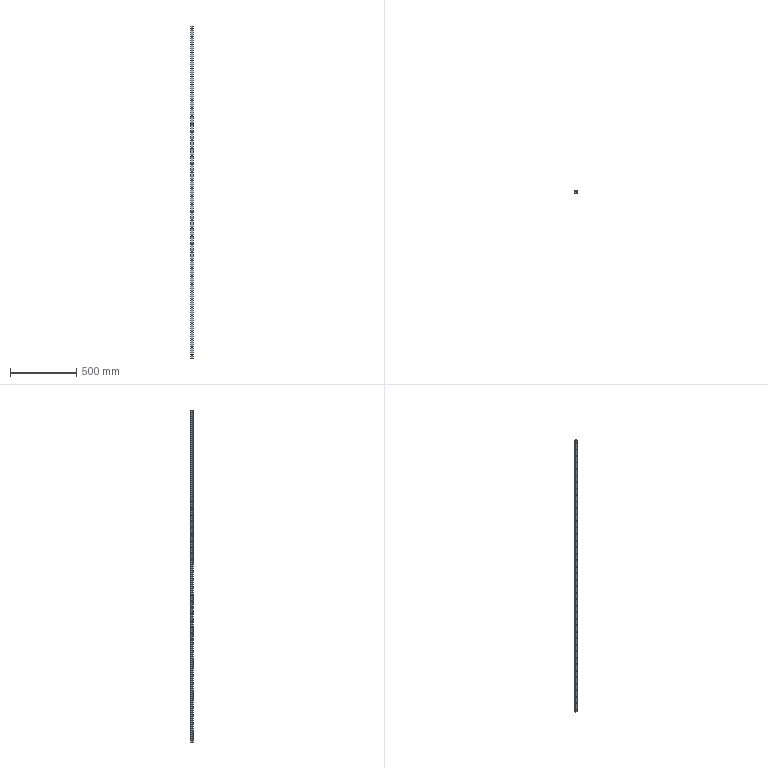Part | STEP file | HGR20-2500 | 1 solid | 254 faces | box 20 x 17.5 x 2500 mm | volume 715425 mm3 | cylinder 190 | plane 64 | commonest cylinder face diameters 6 x84 9.5 x84 1 x12 2 x6 4.06 x4